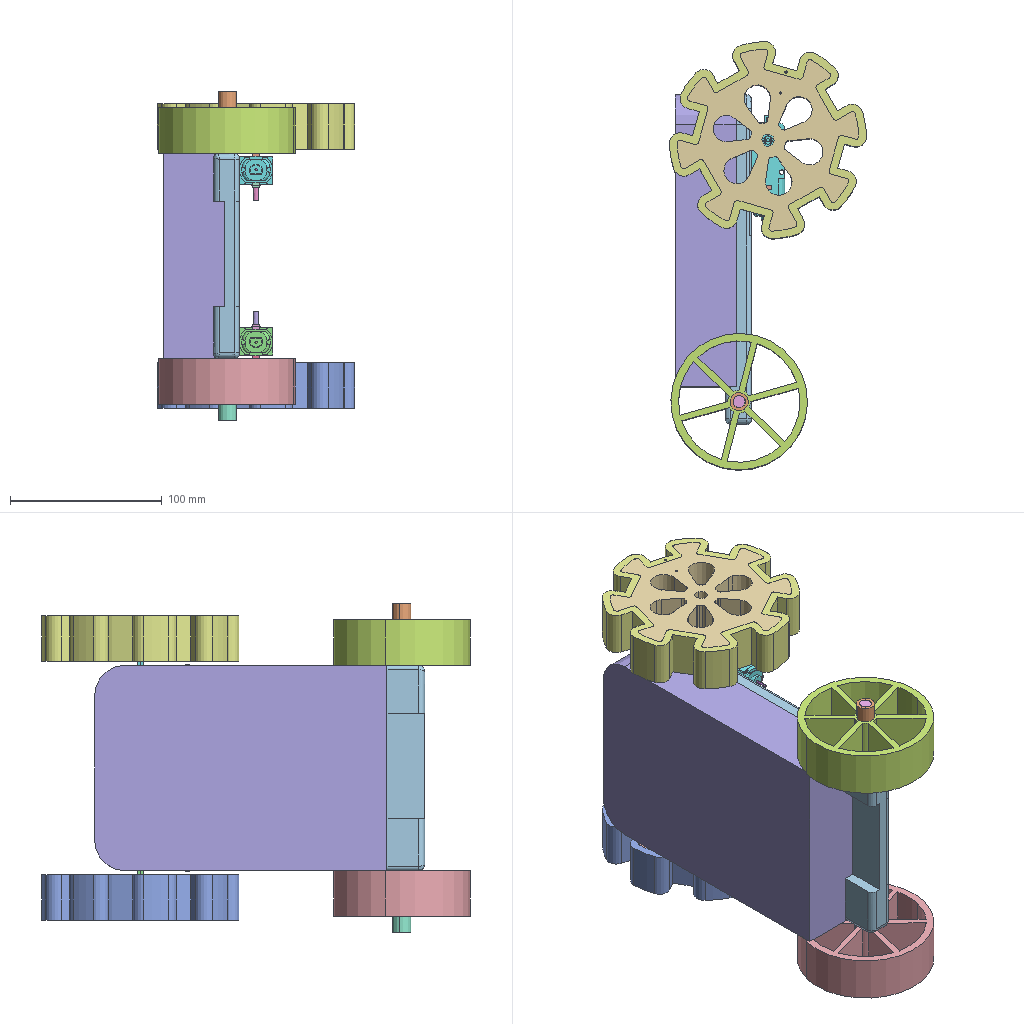Assembly | SolidWorks | 16 different items | 16 placed | box 130 x 282 x 217 mm
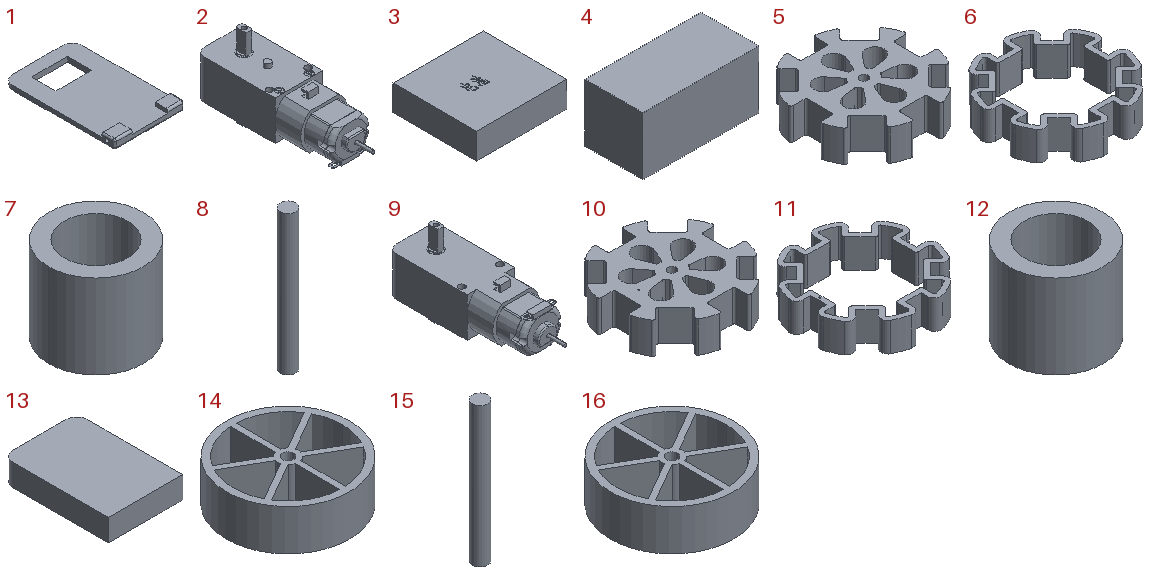Parts list (item | quantity | size | volume | features):
1 | x1 | 135.332 x 217.534 x 17 mm | 263326 mm3 | features ICE 10, Fillet 6, Extrusion 1
2 | x1 | 22 x 77 x 38.5 mm | 22035 mm3 | features ICE 23, Fillet 5, Extrusion 1, RevCut 1
3 | x1 | 70 x 65 x 20 mm | 90986 mm3 | features Extrusion 1, ICE 1
4 | x1 | 60 x 30 x 30 mm | 54000 mm3 | features Extrusion 1
5 | x1 | 117.193 x 117.193 x 30 mm | 181136 mm3 | features ICE 2, CirPattern 1, Extrusion 1, Fillet 1
6 | x1 | 127.193 x 127.193 x 30 mm | 86917 mm3 | features BaseBody 1
7 | x1 | 12 x 12 x 10.677 mm | 657.35 mm3 | features Extrusion 1
8 | x1 | 7.8 x 7.8 x 70 mm | 3345 mm3 | features MirrorStock 1
9 | x1 | 22 x 77 x 38.5 mm | 22035 mm3 | features MirrorStock 1
10 | x1 | 117.193 x 117.193 x 30 mm | 181136 mm3 | features MirrorStock 1
11 | x1 | 127.193 x 127.193 x 30 mm | 86917 mm3 | features MirrorStock 1
12 | x1 | 12 x 12 x 10.677 mm | 657.35 mm3 | features MirrorStock 1
13 | x1 | 135.332 x 192.723 x 40 mm | 238240 mm3 | features Extrusion 1, Shell 1
14 | x1 | 90 x 90 x 30 mm | 67301 mm3 | features BossThin 2, CirPattern 1, Extrusion 1, ICE 1
15 | x1 | 7.8 x 7.8 x 70 mm | 3345 mm3 | features Extrusion 1
16 | x1 | 90 x 90 x 30 mm | 67301 mm3 | features MirrorStock 1
Mates (type | each side: item.copy, entity, surface, feature):
Coincident | 5.1 face plane Boss-Extrude2 | 6.1 face plane Input1 | 3 times
Concentric | 5.1 face cylinder Boss-Extrude2 | 2.1 face cylinder Boss-Extrude12
DistanceDim | 2.1 face plane Boss-Extrude1 | 5.1 face plane Boss-Extrude2
Coincident | 1.1 face plane Boss-Extrude1 | 4.1 face plane Boss-Extrude1
Concentric | 1.1 face cylinder Cut-Extrude5 | 14.1 face cylinder Cut-Extrude1
Coincident | 1.1 face plane Boss-Extrude1 | 14.1 face plane Boss-Extrude1
InPlace | 1.1 face plane Boss-Extrude3 | 15.1 plane
InPlace | 14.1 face plane Boss-Extrude1 | 7.1 plane
InPlace | 1.1 face plane Boss-Extrude1 | 13.1 plane